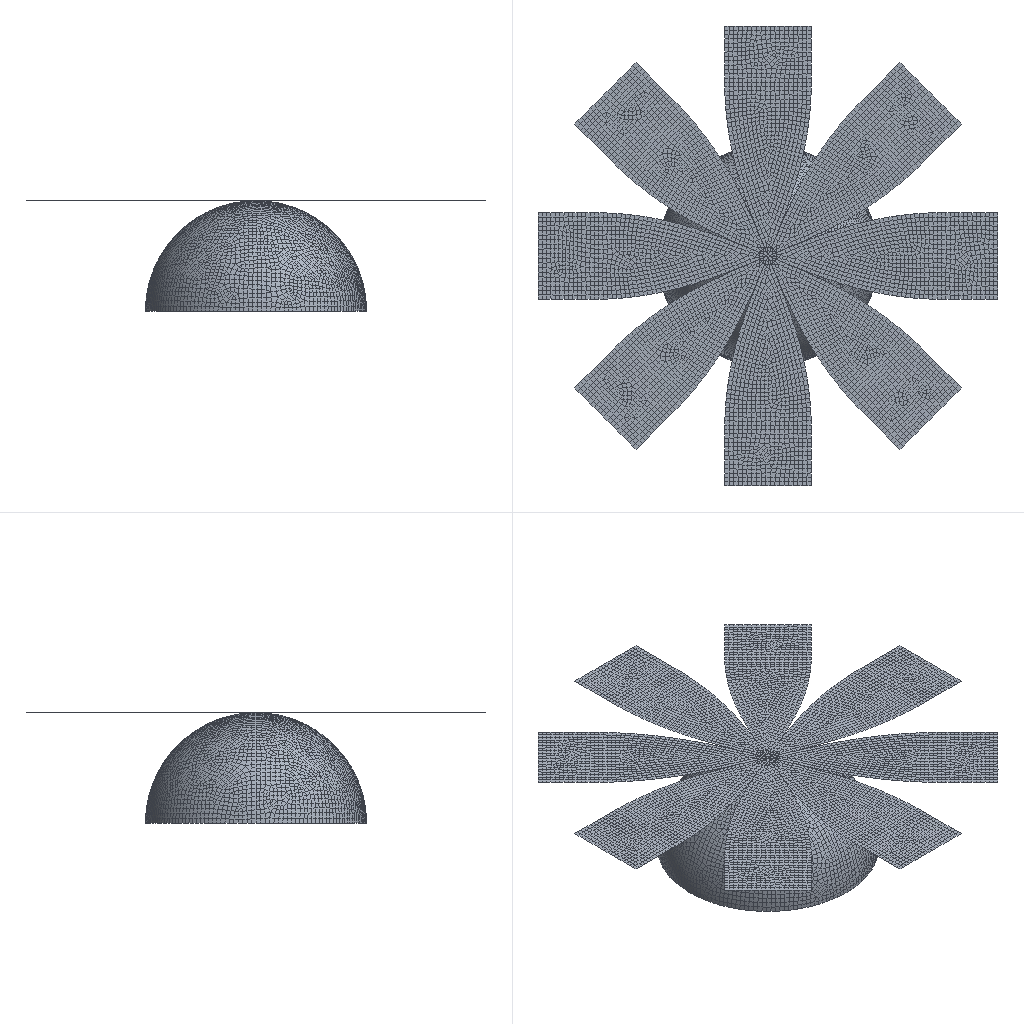Simulation study | abaqus
Set-up summary:
category,name,step,type,value,unit,region
solver,abaqus
solver,version,,,Abaqus/Explicit 2020
units,not stated in the deck,,not stated
analysis,deck,,transient,transient
load_step,Step-1,Step-1,transient,nlgeom=True
contact,interactions,,,general=1 pairs=0 ties=0
load_step,requested,,,1
mesh,nodes,,,11935
mesh,elements,,,11453
element_type,S3,,shell,194
element_type,S4R,,shell,11259
load,load commands in deck,,count,1
bc,support commands in deck,,count,10
material,MATERIAL-1,,in results
material,MATERIAL-2,,in results
check,setup vs results,,match,"per instance, exact: element labels, types and connectivity; labels of the nodes the elements use; coordinates of those nodes at SINGLE_PRECISION in 2 of 2 instance(s)"
Abaqus input file, long lists of numbers shortened:
*Heading
** Job name: Job-2 Model name: Model-1-Copy
** Generated by: Abaqus/CAE 2020
*Preprint, echo=NO, model=NO, history=NO, contact=NO
**
** PARTS
**
*Part, name=final
*Node
      1,   4.84,  -19.362, -3.42691607e-07
      2,  -4.84,  -19.362, -3.4269155e-07
** (7227 more lines like these left out)
*Element, type=S3
1, 1619, 1583, 1582
2, 1650, 1634, 1639
** (32 more lines like these left out)
*Element, type=S4R
  4, 1230, 1241, 1167, 1138
  5,  126, 1156, 1191,  125
** (6709 more lines like these left out)
*Nset, nset=Set-1, generate
    1,  7229,     1
*Elset, elset=Set-1, generate
    1,  6745,     1
** Section: Section-1
*Shell Section, elset=Set-1, material=Material-1
0.266, 5
*End Part
**
*Part, name=work-1
*Node
      1,  -303.738,  -125.23,  -266.987
      2,  -291.408,  -125.23,  -254.657
** (4704 more lines like these left out)
*Element, type=S3
 1,  292,  319,  288
 2,  881, 2355,  880
** (158 more lines like these left out)
*Element, type=S4R
  92,  270,  156,    1,    5
  93,  272,  155,  156,  270
** (4546 more lines like these left out)
*Nset, nset=Set-1, generate
    1,  4706,     1
*Elset, elset=Set-1, generate
    1,  4708,     1
** Section: Section-2
*Shell Section, elset=Set-1, material=Material-2
1., 5
*End Part
**
**
** ASSEMBLY
**
*Assembly, name=Assembly
**
*Instance, name=work-1-1, part=work-1
  291.408,   125.23,   254.657
*End Instance
**
*Instance, name=final-1, part=final
*End Instance
**
*Node
      1, 2.13960163e-07, 2.81027724e-07,  -12.33
*Nset, nset=Set-1, instance=final-1
    1,    2,    4,    5,    6,    7,    8,    9,   10,   11,   12,   13,   14,   15,   16,   17
   18,   19,   20,   21,   22,   23,   24,   25,   26,   27,   28,   29,   30,   31,   32,   33
** (150 more lines like these left out)
*Elset, elset=Set-1, instance=final-1
  571,  572,  573,  574,  575,  576,  577,  578,  579,  580,  581,  582,  583,  584,  585,  586
  587,  588,  589,  590,  591,  592,  593,  594,  595,  596,  597,  598,  599,  600,  601,  602
** (133 more lines like these left out)
*Nset, nset=Set-4
 1,
*Nset, nset=Set-5, instance=final-1
    1,    2,    4,    5,    6,    7,    8,    9,   10,   11,   12,   13,   14,   15,   16,   17
   18,   19,   20,   21,   22,   23,   24,   25,   26,   27,   28,   29,   30,   31,   32,   33
** (150 more lines like these left out)
*Elset, elset=Set-5, instance=final-1
  571,  572,  573,  574,  575,  576,  577,  578,  579,  580,  581,  582,  583,  584,  585,  586
  587,  588,  589,  590,  591,  592,  593,  594,  595,  596,  597,  598,  599,  600,  601,  602
** (133 more lines like these left out)
*Nset, nset=b_Set-2, instance=work-1-1, generate
    1,  4706,     1
*Elset, elset=b_Set-2, instance=work-1-1, generate
    1,  4708,     1
*Nset, nset=_PickedSet55, internal
 1,
** Constraint: Constraint-1
*Rigid Body, ref node=_PickedSet55, elset=b_Set-2
*End Assembly
*Amplitude, name=Amp-1
             0.,              0.,              1.,              1.
**
** MATERIALS
**
*Material, name=Material-1
*Density
 1.0593e-09,
*Elastic
 2.6, 0.47
*Material, name=Material-2
*Density
 7.8e-09,
*Elastic
210000., 0.3
**
** INTERACTION PROPERTIES
**
*Surface Interaction, name=IntProp-1
*Friction
 0.1,
*Surface Behavior, pressure-overclosure=HARD
**
** INTERACTIONS
**
** Interaction: Int-2
*Contact, op=NEW
*Contact Inclusions, ALL EXTERIOR
*Contact Property Assignment
 ,  , IntProp-1
** ----------------------------------------------------------------
**
** STEP: Step-1
**
*Step, name=Step-1, nlgeom=YES
*Dynamic, Explicit
, 1.
*Bulk Viscosity
0.06, 1.2
**
** BOUNDARY CONDITIONS
**
** Name: BC-1 Type: 位移/转角
*Boundary
Set-5, 3, 3
Set-5, 4, 4
Set-5, 5, 5
Set-5, 6, 6
** Name: [REDACTED] : Displacement/rotation angle
*Boundary, amplitude=Amp-1
Set-4, 1, 1
Set-4, 2, 2
Set-4, 3, 3, 12.
Set-4, 4, 4
Set-4, 5, 5
Set-4, 6, 6
**
** OUTPUT REQUESTS
**
*Restart, write, number interval=1, time marks=NO
**
** FIELD OUTPUT: F-Output-1
**
*Output, field
*Node Output
CF, RF, RM, RT, U, V
*Element Output, directions=YES
E, LE, MISES, MISESMAX, MISESONLY, NE, PE, PEEQ, PEEQMAX, PEEQT, PEMAG, PRESSONLY, S, SEQUT, SF, SSAVG
YIELDPOT
*Contact Output
CDISP, CFORCE, CSTRESS, PPRESS
**
** HISTORY OUTPUT: H-Output-1
**
*Output, history, variable=PRESELECT
*End Step
Results summary:
result,step,Step-1,completed,increments=294466 time=1.0/1.0
result,analysis,,,transient
result,last_loadstep,,,1
result,analysis steps,,count,1
result,primary field,,,"U, UR"
result,reaction total,,FX,-0.001881,model units
result,reaction total,,FY,-0.000244,model units
result,reaction total,,FZ,0.004044,model units